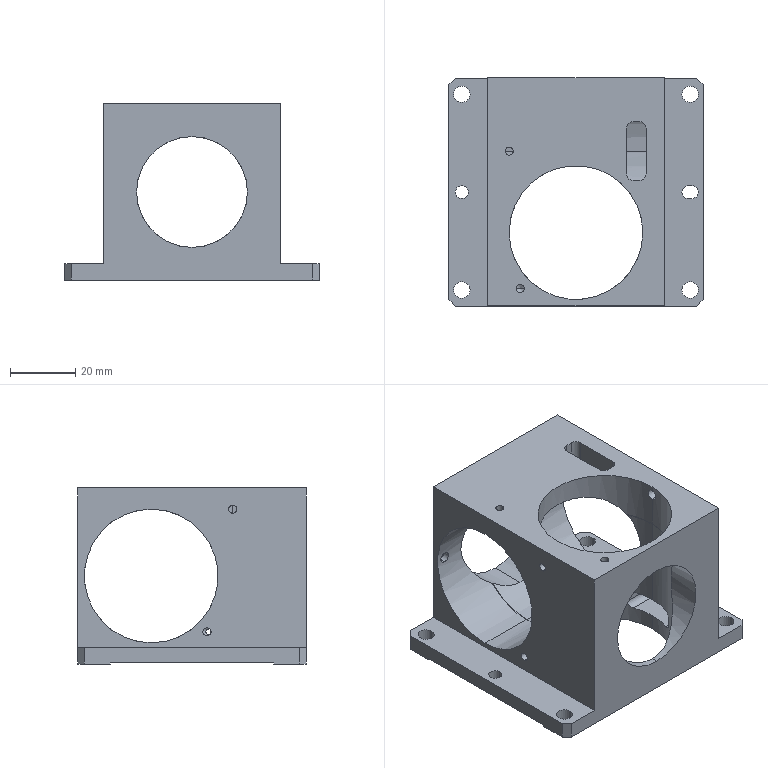NC program | NX | posted with a generic post | part box 78 x 70 x 54 mm
Lines 1 to 33 of 5040:
N10 G17 G21 G94 G90
(FLOOR_WALL , TOOL : D63)
N12 T01 M6
N14 G54
N16 G17 G0 G90 X-75.5 Y36.997 B0. C0. S6500 M3
N18 G43 Z30. H1
N20 Z3.
N22 G94 G1 Z0. F1500.
N24 X-72.5
N26 X72.5
N28 Y-11.8
N30 X-72.5
N32 X-75.5
N34 Z3.
N36 G0 Z30.
N38 M5
(DRILLING , TOOL : D6A45)
N40 T07 M6
N42 G54
N44 G17 G0 G90 X-17.1 Y-29.6 B0. C0. S5000 M3
N46 G43 Z30. H7
N48 G94 G81 G98 Z-1.6 F250. R3.
N50 X0. Y-12.5
N52 X-20.5 Y12.5
N54 G80
N56 G0 X-20.5 Y12.5 Z30.
N58 M5